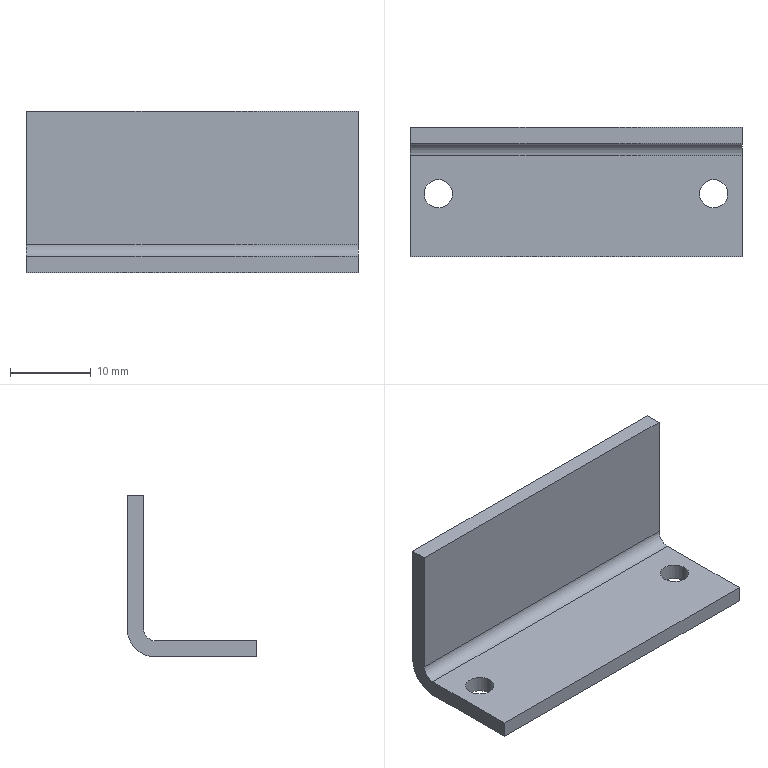Part | SolidWorks | features BaseBody 1 | 1 solid | 14 faces | box 41 x 16 x 20 mm | volume 2662 mm3 | plane 8 | cylinder 6 | commonest cylinder face diameters 3.5 x4 3 x1 7 x1
STEP:
#1=CARTESIAN_POINT('',(-15.25,-0.2,0.));
#2=VERTEX_POINT('',#1);
#3=CARTESIAN_POINT('',(-18.75,-0.2,0.));
#4=VERTEX_POINT('',#3);
#5=CARTESIAN_POINT('',(-17.,-0.2,0.));
#6=DIRECTION('',(0.,0.,-1.));
#7=DIRECTION('',(-1.,0.,0.));
#8=AXIS2_PLACEMENT_3D('',#5,#6,#7);
#9=CIRCLE('',#8,1.75);
#10=EDGE_CURVE('',#2,#4,#9,.T.);
#11=ORIENTED_EDGE('',*,*,#10,.F.);
#12=CARTESIAN_POINT('',(-15.25,-0.2,-2.));
#13=VERTEX_POINT('',#12);
#14=CARTESIAN_POINT('',(-15.25,-0.2,8.));
#15=DIRECTION('',(0.,0.,-1.));
#16=VECTOR('',#15,1000.);
#17=LINE('',#14,#16);
#18=EDGE_CURVE('',#2,#13,#17,.T.);
#19=ORIENTED_EDGE('',*,*,#18,.T.);
#20=CARTESIAN_POINT('',(-18.75,-0.2,-2.));
#21=VERTEX_POINT('',#20);
#22=CARTESIAN_POINT('',(-17.,-0.2,-2.));
#23=DIRECTION('',(0.,0.,1.));
#24=DIRECTION('',(-1.,0.,0.));
#25=AXIS2_PLACEMENT_3D('',#22,#23,#24);
#26=CIRCLE('',#25,1.75);
#27=EDGE_CURVE('',#21,#13,#26,.T.);
#28=ORIENTED_EDGE('',*,*,#27,.F.);
#29=CARTESIAN_POINT('',(-18.75,-0.2,8.));
#30=DIRECTION('',(0.,0.,-1.));
#31=VECTOR('',#30,1000.);
#32=LINE('',#29,#31);
#33=EDGE_CURVE('',#4,#21,#32,.T.);
#34=ORIENTED_EDGE('',*,*,#33,.F.);
#35=EDGE_LOOP('',(#11,#19,#28,#34));
#36=FACE_OUTER_BOUND('',#35,.T.);
#37=CARTESIAN_POINT('',(-17.,-0.2,8.));
#38=DIRECTION('',(0.,0.,-1.));
#39=DIRECTION('',(-1.,0.,0.));
#40=AXIS2_PLACEMENT_3D('',#37,#38,#39);
#41=CYLINDRICAL_SURFACE('',#40,1.75);
#42=ADVANCED_FACE('',(#36),#41,.F.);
#43=CARTESIAN_POINT('',(18.75,-0.2,0.));
#44=VERTEX_POINT('',#43);
#45=CARTESIAN_POINT('',(15.25,-0.2,0.));
#46=VERTEX_POINT('',#45);
#47=CARTESIAN_POINT('',(17.,-0.2,0.));
#48=DIRECTION('',(0.,0.,-1.));
#49=DIRECTION('',(-1.,0.,0.));
#50=AXIS2_PLACEMENT_3D('',#47,#48,#49);
#51=CIRCLE('',#50,1.75);
#52=EDGE_CURVE('',#44,#46,#51,.T.);
#53=ORIENTED_EDGE('',*,*,#52,.F.);
#54=CARTESIAN_POINT('',(18.75,-0.2,-2.));
#55=VERTEX_POINT('',#54);
#56=CARTESIAN_POINT('',(18.75,-0.2,8.));
#57=DIRECTION('',(0.,0.,-1.));
#58=VECTOR('',#57,1000.);
#59=LINE('',#56,#58);
#60=EDGE_CURVE('',#44,#55,#59,.T.);
#61=ORIENTED_EDGE('',*,*,#60,.T.);
#62=CARTESIAN_POINT('',(15.25,-0.2,-2.));
#63=VERTEX_POINT('',#62);
#64=CARTESIAN_POINT('',(17.,-0.2,-2.));
#65=DIRECTION('',(0.,0.,1.));
#66=DIRECTION('',(-1.,0.,0.));
#67=AXIS2_PLACEMENT_3D('',#64,#65,#66);
#68=CIRCLE('',#67,1.75);
#69=EDGE_CURVE('',#63,#55,#68,.T.);
#70=ORIENTED_EDGE('',*,*,#69,.F.);
#71=CARTESIAN_POINT('',(15.25,-0.2,8.));
#72=DIRECTION('',(0.,0.,-1.));
#73=VECTOR('',#72,1000.);
#74=LINE('',#71,#73);
#75=EDGE_CURVE('',#46,#63,#74,.T.);
#76=ORIENTED_EDGE('',*,*,#75,.F.);
#77=EDGE_LOOP('',(#53,#61,#70,#76));
#78=FACE_OUTER_BOUND('',#77,.T.);
#79=CARTESIAN_POINT('',(17.,-0.2,8.));
#80=DIRECTION('',(0.,0.,-1.));
#81=DIRECTION('',(-1.,0.,0.));
#82=AXIS2_PLACEMENT_3D('',#79,#80,#81);
#83=CYLINDRICAL_SURFACE('',#82,1.75);
#84=ADVANCED_FACE('',(#78),#83,.F.);
#85=CARTESIAN_POINT('',(-20.5,8.,1.5));
#86=VERTEX_POINT('',#85);
#87=CARTESIAN_POINT('',(-20.5,8.,18.));
#88=VERTEX_POINT('',#87);
#89=CARTESIAN_POINT('',(-20.5,8.,0.));
#90=DIRECTION('',(0.,0.,1.));
#91=VECTOR('',#90,1000.);
#92=LINE('',#89,#91);
#93=EDGE_CURVE('',#86,#88,#92,.T.);
#94=ORIENTED_EDGE('',*,*,#93,.T.);
#95=CARTESIAN_POINT('',(20.5,8.,18.));
#96=VERTEX_POINT('',#95);
#97=CARTESIAN_POINT('',(0.,8.,18.));
#98=DIRECTION('',(1.,0.,0.));
#99=VECTOR('',#98,1000.);
#100=LINE('',#97,#99);
#101=EDGE_CURVE('',#88,#96,#100,.T.);
#102=ORIENTED_EDGE('',*,*,#101,.T.);
#103=CARTESIAN_POINT('',(20.5,8.,1.5));
#104=VERTEX_POINT('',#103);
#105=CARTESIAN_POINT('',(20.5,8.,0.));
#106=DIRECTION('',(0.,0.,-1.));
#107=VECTOR('',#106,1000.);
#108=LINE('',#105,#107);
#109=EDGE_CURVE('',#96,#104,#108,.T.);
#110=ORIENTED_EDGE('',*,*,#109,.T.);
#111=CARTESIAN_POINT('',(0.,8.,1.5));
#112=DIRECTION('',(-1.,0.,0.));
#113=VECTOR('',#112,1000.);
#114=LINE('',#111,#113);
#115=EDGE_CURVE('',#104,#86,#114,.T.);
#116=ORIENTED_EDGE('',*,*,#115,.T.);
#117=EDGE_LOOP('',(#94,#102,#110,#116));
#118=FACE_OUTER_BOUND('',#117,.T.);
#119=CARTESIAN_POINT('',(0.,8.,0.));
#120=DIRECTION('',(0.,1.,0.));
#121=DIRECTION('',(0.,0.,1.));
#122=AXIS2_PLACEMENT_3D('',#119,#120,#121);
#123=PLANE('',#122);
#124=ADVANCED_FACE('',(#118),#123,.T.);
#125=ORIENTED_EDGE('',*,*,#101,.F.);
#126=CARTESIAN_POINT('',(-20.5,6.,18.));
#127=VERTEX_POINT('',#126);
#128=CARTESIAN_POINT('',(-20.5,8.,18.));
#129=DIRECTION('',(0.,-1.,0.));
#130=VECTOR('',#129,1000.);
#131=LINE('',#128,#130);
#132=EDGE_CURVE('',#88,#127,#131,.T.);
#133=ORIENTED_EDGE('',*,*,#132,.T.);
#134=CARTESIAN_POINT('',(20.5,6.,18.));
#135=VERTEX_POINT('',#134);
#136=CARTESIAN_POINT('',(-20.5,6.,18.));
#137=DIRECTION('',(1.,0.,0.));
#138=VECTOR('',#137,1000.);
#139=LINE('',#136,#138);
#140=EDGE_CURVE('',#127,#135,#139,.T.);
#141=ORIENTED_EDGE('',*,*,#140,.T.);
#142=CARTESIAN_POINT('',(20.5,8.,18.));
#143=DIRECTION('',(0.,1.,0.));
#144=VECTOR('',#143,1000.);
#145=LINE('',#142,#144);
#146=EDGE_CURVE('',#135,#96,#145,.T.);
#147=ORIENTED_EDGE('',*,*,#146,.T.);
#148=EDGE_LOOP('',(#125,#133,#141,#147));
#149=FACE_OUTER_BOUND('',#148,.T.);
#150=CARTESIAN_POINT('',(-20.5,8.,18.));
#151=DIRECTION('',(0.,0.,1.));
#152=DIRECTION('',(0.,-1.,0.));
#153=AXIS2_PLACEMENT_3D('',#150,#151,#152);
#154=PLANE('',#153);
#155=ADVANCED_FACE('',(#149),#154,.T.);
#156=CARTESIAN_POINT('',(-20.5,6.,1.5));
#157=VERTEX_POINT('',#156);
#158=CARTESIAN_POINT('',(-20.5,6.,0.));
#159=DIRECTION('',(0.,0.,1.));
#160=VECTOR('',#159,1000.);
#161=LINE('',#158,#160);
#162=EDGE_CURVE('',#157,#127,#161,.T.);
#163=ORIENTED_EDGE('',*,*,#162,.T.);
#164=ORIENTED_EDGE('',*,*,#132,.F.);
#165=ORIENTED_EDGE('',*,*,#93,.F.);
#166=CARTESIAN_POINT('',(-20.5,4.5,-2.));
#167=VERTEX_POINT('',#166);
#168=CARTESIAN_POINT('',(-20.5,4.5,1.5));
#169=DIRECTION('',(1.,0.,0.));
#170=DIRECTION('',(0.,0.,1.));
#171=AXIS2_PLACEMENT_3D('',#168,#169,#170);
#172=CIRCLE('',#171,3.5);
#173=EDGE_CURVE('',#167,#86,#172,.T.);
#174=ORIENTED_EDGE('',*,*,#173,.F.);
#175=CARTESIAN_POINT('',(-20.5,-8.,-2.));
#176=VERTEX_POINT('',#175);
#177=CARTESIAN_POINT('',(-20.5,0.,-2.));
#178=DIRECTION('',(0.,1.,0.));
#179=VECTOR('',#178,1000.);
#180=LINE('',#177,#179);
#181=EDGE_CURVE('',#176,#167,#180,.T.);
#182=ORIENTED_EDGE('',*,*,#181,.F.);
#183=CARTESIAN_POINT('',(-20.5,-8.,0.));
#184=VERTEX_POINT('',#183);
#185=CARTESIAN_POINT('',(-20.5,-8.,-2.));
#186=DIRECTION('',(0.,0.,1.));
#187=VECTOR('',#186,1000.);
#188=LINE('',#185,#187);
#189=EDGE_CURVE('',#176,#184,#188,.T.);
#190=ORIENTED_EDGE('',*,*,#189,.T.);
#191=CARTESIAN_POINT('',(-20.5,4.5,0.));
#192=VERTEX_POINT('',#191);
#193=CARTESIAN_POINT('',(-20.5,-8.,0.));
#194=DIRECTION('',(0.,1.,0.));
#195=VECTOR('',#194,1000.);
#196=LINE('',#193,#195);
#197=EDGE_CURVE('',#184,#192,#196,.T.);
#198=ORIENTED_EDGE('',*,*,#197,.T.);
#199=CARTESIAN_POINT('',(-20.5,4.5,1.5));
#200=DIRECTION('',(-1.,0.,0.));
#201=DIRECTION('',(0.,0.,1.));
#202=AXIS2_PLACEMENT_3D('',#199,#200,#201);
#203=CIRCLE('',#202,1.5);
#204=EDGE_CURVE('',#157,#192,#203,.T.);
#205=ORIENTED_EDGE('',*,*,#204,.F.);
#206=EDGE_LOOP('',(#163,#164,#165,#174,#182,#190,#198,#205));
#207=FACE_OUTER_BOUND('',#206,.T.);
#208=CARTESIAN_POINT('',(-20.5,8.,0.));
#209=DIRECTION('',(-1.,0.,0.));
#210=DIRECTION('',(0.,0.,1.));
#211=AXIS2_PLACEMENT_3D('',#208,#209,#210);
#212=PLANE('',#211);
#213=ADVANCED_FACE('',(#207),#212,.T.);
#214=ORIENTED_EDGE('',*,*,#115,.F.);
#215=CARTESIAN_POINT('',(20.5,4.5,-2.));
#216=VERTEX_POINT('',#215);
#217=CARTESIAN_POINT('',(20.5,4.5,1.5));
#218=DIRECTION('',(-1.,0.,0.));
#219=DIRECTION('',(0.,0.,1.));
#220=AXIS2_PLACEMENT_3D('',#217,#218,#219);
#221=CIRCLE('',#220,3.5);
#222=EDGE_CURVE('',#104,#216,#221,.T.);
#223=ORIENTED_EDGE('',*,*,#222,.T.);
#224=CARTESIAN_POINT('',(-20.5,4.5,-2.));
#225=DIRECTION('',(-1.,0.,0.));
#226=VECTOR('',#225,1000.);
#227=LINE('',#224,#226);
#228=EDGE_CURVE('',#216,#167,#227,.T.);
#229=ORIENTED_EDGE('',*,*,#228,.T.);
#230=ORIENTED_EDGE('',*,*,#173,.T.);
#231=EDGE_LOOP('',(#214,#223,#229,#230));
#232=FACE_OUTER_BOUND('',#231,.T.);
#233=CARTESIAN_POINT('',(-20.5,4.5,1.5));
#234=DIRECTION('',(-1.,0.,0.));
#235=DIRECTION('',(0.,0.,1.));
#236=AXIS2_PLACEMENT_3D('',#233,#234,#235);
#237=CYLINDRICAL_SURFACE('',#236,3.5);
#238=ADVANCED_FACE('',(#232),#237,.T.);
#239=ORIENTED_EDGE('',*,*,#109,.F.);
#240=ORIENTED_EDGE('',*,*,#146,.F.);
#241=CARTESIAN_POINT('',(20.5,6.,1.5));
#242=VERTEX_POINT('',#241);
#243=CARTESIAN_POINT('',(20.5,6.,18.));
#244=DIRECTION('',(0.,0.,-1.));
#245=VECTOR('',#244,1000.);
#246=LINE('',#243,#245);
#247=EDGE_CURVE('',#135,#242,#246,.T.);
#248=ORIENTED_EDGE('',*,*,#247,.T.);
#249=CARTESIAN_POINT('',(20.5,4.5,0.));
#250=VERTEX_POINT('',#249);
#251=CARTESIAN_POINT('',(20.5,4.5,1.5));
#252=DIRECTION('',(-1.,0.,0.));
#253=DIRECTION('',(0.,0.,1.));
#254=AXIS2_PLACEMENT_3D('',#251,#252,#253);
#255=CIRCLE('',#254,1.5);
#256=EDGE_CURVE('',#242,#250,#255,.T.);
#257=ORIENTED_EDGE('',*,*,#256,.T.);
#258=CARTESIAN_POINT('',(20.5,-8.,0.));
#259=VERTEX_POINT('',#258);
#260=CARTESIAN_POINT('',(20.5,-8.,0.));
#261=DIRECTION('',(0.,-1.,0.));
#262=VECTOR('',#261,1000.);
#263=LINE('',#260,#262);
#264=EDGE_CURVE('',#250,#259,#263,.T.);
#265=ORIENTED_EDGE('',*,*,#264,.T.);
#266=CARTESIAN_POINT('',(20.5,-8.,-2.));
#267=VERTEX_POINT('',#266);
#268=CARTESIAN_POINT('',(20.5,-8.,-2.));
#269=DIRECTION('',(0.,0.,-1.));
#270=VECTOR('',#269,1000.);
#271=LINE('',#268,#270);
#272=EDGE_CURVE('',#259,#267,#271,.T.);
#273=ORIENTED_EDGE('',*,*,#272,.T.);
#274=CARTESIAN_POINT('',(20.5,0.,-2.));
#275=DIRECTION('',(0.,-1.,0.));
#276=VECTOR('',#275,1000.);
#277=LINE('',#274,#276);
#278=EDGE_CURVE('',#216,#267,#277,.T.);
#279=ORIENTED_EDGE('',*,*,#278,.F.);
#280=ORIENTED_EDGE('',*,*,#222,.F.);
#281=EDGE_LOOP('',(#239,#240,#248,#257,#265,#273,#279,#280));
#282=FACE_OUTER_BOUND('',#281,.T.);
#283=CARTESIAN_POINT('',(20.5,8.,18.));
#284=DIRECTION('',(1.,0.,0.));
#285=DIRECTION('',(0.,0.,-1.));
#286=AXIS2_PLACEMENT_3D('',#283,#284,#285);
#287=PLANE('',#286);
#288=ADVANCED_FACE('',(#282),#287,.T.);
#289=ORIENTED_EDGE('',*,*,#247,.F.);
#290=ORIENTED_EDGE('',*,*,#140,.F.);
#291=ORIENTED_EDGE('',*,*,#162,.F.);
#292=CARTESIAN_POINT('',(0.,6.,1.5));
#293=DIRECTION('',(-1.,0.,0.));
#294=VECTOR('',#293,1000.);
#295=LINE('',#292,#294);
#296=EDGE_CURVE('',#242,#157,#295,.T.);
#297=ORIENTED_EDGE('',*,*,#296,.F.);
#298=EDGE_LOOP('',(#289,#290,#291,#297));
#299=FACE_OUTER_BOUND('',#298,.T.);
#300=CARTESIAN_POINT('',(0.,6.,0.));
#301=DIRECTION('',(0.,1.,0.));
#302=DIRECTION('',(0.,0.,1.));
#303=AXIS2_PLACEMENT_3D('',#300,#301,#302);
#304=PLANE('',#303);
#305=ADVANCED_FACE('',(#299),#304,.F.);
#306=ORIENTED_EDGE('',*,*,#278,.T.);
#307=CARTESIAN_POINT('',(0.,-8.,-2.));
#308=DIRECTION('',(-1.,0.,0.));
#309=VECTOR('',#308,1000.);
#310=LINE('',#307,#309);
#311=EDGE_CURVE('',#267,#176,#310,.T.);
#312=ORIENTED_EDGE('',*,*,#311,.T.);
#313=ORIENTED_EDGE('',*,*,#181,.T.);
#314=ORIENTED_EDGE('',*,*,#228,.F.);
#315=EDGE_LOOP('',(#306,#312,#313,#314));
#316=FACE_OUTER_BOUND('',#315,.T.);
#317=ORIENTED_EDGE('',*,*,#27,.T.);
#318=CARTESIAN_POINT('',(-17.,-0.2,-2.));
#319=DIRECTION('',(0.,0.,1.));
#320=DIRECTION('',(-1.,0.,0.));
#321=AXIS2_PLACEMENT_3D('',#318,#319,#320);
#322=CIRCLE('',#321,1.75);
#323=EDGE_CURVE('',#13,#21,#322,.T.);
#324=ORIENTED_EDGE('',*,*,#323,.T.);
#325=EDGE_LOOP('',(#317,#324));
#326=FACE_BOUND('',#325,.T.);
#327=ORIENTED_EDGE('',*,*,#69,.T.);
#328=CARTESIAN_POINT('',(17.,-0.2,-2.));
#329=DIRECTION('',(0.,0.,1.));
#330=DIRECTION('',(-1.,0.,0.));
#331=AXIS2_PLACEMENT_3D('',#328,#329,#330);
#332=CIRCLE('',#331,1.75);
#333=EDGE_CURVE('',#55,#63,#332,.T.);
#334=ORIENTED_EDGE('',*,*,#333,.T.);
#335=EDGE_LOOP('',(#327,#334));
#336=FACE_BOUND('',#335,.T.);
#337=CARTESIAN_POINT('',(0.,0.,-2.));
#338=DIRECTION('',(0.,0.,-1.));
#339=DIRECTION('',(-1.,0.,0.));
#340=AXIS2_PLACEMENT_3D('',#337,#338,#339);
#341=PLANE('',#340);
#342=ADVANCED_FACE('',(#316,#326,#336),#341,.T.);
#343=ORIENTED_EDGE('',*,*,#256,.F.);
#344=ORIENTED_EDGE('',*,*,#296,.T.);
#345=ORIENTED_EDGE('',*,*,#204,.T.);
#346=CARTESIAN_POINT('',(-20.5,4.5,0.));
#347=DIRECTION('',(-1.,0.,0.));
#348=VECTOR('',#347,1000.);
#349=LINE('',#346,#348);
#350=EDGE_CURVE('',#250,#192,#349,.T.);
#351=ORIENTED_EDGE('',*,*,#350,.F.);
#352=EDGE_LOOP('',(#343,#344,#345,#351));
#353=FACE_OUTER_BOUND('',#352,.T.);
#354=CARTESIAN_POINT('',(-20.5,4.5,1.5));
#355=DIRECTION('',(-1.,0.,0.));
#356=DIRECTION('',(0.,0.,1.));
#357=AXIS2_PLACEMENT_3D('',#354,#355,#356);
#358=CYLINDRICAL_SURFACE('',#357,1.5);
#359=ADVANCED_FACE('',(#353),#358,.F.);
#360=ORIENTED_EDGE('',*,*,#311,.F.);
#361=ORIENTED_EDGE('',*,*,#272,.F.);
#362=CARTESIAN_POINT('',(-20.5,-8.,0.));
#363=DIRECTION('',(-1.,0.,0.));
#364=VECTOR('',#363,1000.);
#365=LINE('',#362,#364);
#366=EDGE_CURVE('',#259,#184,#365,.T.);
#367=ORIENTED_EDGE('',*,*,#366,.T.);
#368=ORIENTED_EDGE('',*,*,#189,.F.);
#369=EDGE_LOOP('',(#360,#361,#367,#368));
#370=FACE_OUTER_BOUND('',#369,.T.);
#371=CARTESIAN_POINT('',(-20.5,-8.,-2.));
#372=DIRECTION('',(0.,-1.,0.));
#373=DIRECTION('',(0.,0.,-1.));
#374=AXIS2_PLACEMENT_3D('',#371,#372,#373);
#375=PLANE('',#374);
#376=ADVANCED_FACE('',(#370),#375,.T.);
#377=ORIENTED_EDGE('',*,*,#18,.F.);
#378=CARTESIAN_POINT('',(-17.,-0.2,0.));
#379=DIRECTION('',(0.,0.,-1.));
#380=DIRECTION('',(-1.,0.,0.));
#381=AXIS2_PLACEMENT_3D('',#378,#379,#380);
#382=CIRCLE('',#381,1.75);
#383=EDGE_CURVE('',#4,#2,#382,.T.);
#384=ORIENTED_EDGE('',*,*,#383,.F.);
#385=ORIENTED_EDGE('',*,*,#33,.T.);
#386=ORIENTED_EDGE('',*,*,#323,.F.);
#387=EDGE_LOOP('',(#377,#384,#385,#386));
#388=FACE_OUTER_BOUND('',#387,.T.);
#389=CARTESIAN_POINT('',(-17.,-0.2,8.));
#390=DIRECTION('',(0.,0.,-1.));
#391=DIRECTION('',(-1.,0.,0.));
#392=AXIS2_PLACEMENT_3D('',#389,#390,#391);
#393=CYLINDRICAL_SURFACE('',#392,1.75);
#394=ADVANCED_FACE('',(#388),#393,.F.);
#395=ORIENTED_EDGE('',*,*,#60,.F.);
#396=CARTESIAN_POINT('',(17.,-0.2,0.));
#397=DIRECTION('',(0.,0.,-1.));
#398=DIRECTION('',(-1.,0.,0.));
#399=AXIS2_PLACEMENT_3D('',#396,#397,#398);
#400=CIRCLE('',#399,1.75);
#401=EDGE_CURVE('',#46,#44,#400,.T.);
#402=ORIENTED_EDGE('',*,*,#401,.F.);
#403=ORIENTED_EDGE('',*,*,#75,.T.);
#404=ORIENTED_EDGE('',*,*,#333,.F.);
#405=EDGE_LOOP('',(#395,#402,#403,#404));
#406=FACE_OUTER_BOUND('',#405,.T.);
#407=CARTESIAN_POINT('',(17.,-0.2,8.));
#408=DIRECTION('',(0.,0.,-1.));
#409=DIRECTION('',(-1.,0.,0.));
#410=AXIS2_PLACEMENT_3D('',#407,#408,#409);
#411=CYLINDRICAL_SURFACE('',#410,1.75);
#412=ADVANCED_FACE('',(#406),#411,.F.);
#413=ORIENTED_EDGE('',*,*,#197,.F.);
#414=ORIENTED_EDGE('',*,*,#366,.F.);
#415=ORIENTED_EDGE('',*,*,#264,.F.);
#416=ORIENTED_EDGE('',*,*,#350,.T.);
#417=EDGE_LOOP('',(#413,#414,#415,#416));
#418=FACE_OUTER_BOUND('',#417,.T.);
#419=ORIENTED_EDGE('',*,*,#383,.T.);
#420=ORIENTED_EDGE('',*,*,#10,.T.);
#421=EDGE_LOOP('',(#419,#420));
#422=FACE_BOUND('',#421,.T.);
#423=ORIENTED_EDGE('',*,*,#401,.T.);
#424=ORIENTED_EDGE('',*,*,#52,.T.);
#425=EDGE_LOOP('',(#423,#424));
#426=FACE_BOUND('',#425,.T.);
#427=CARTESIAN_POINT('',(0.,0.,0.));
#428=DIRECTION('',(0.,0.,-1.));
#429=DIRECTION('',(-1.,0.,0.));
#430=AXIS2_PLACEMENT_3D('',#427,#428,#429);
#431=PLANE('',#430);
#432=ADVANCED_FACE('',(#418,#422,#426),#431,.F.);
#433=CLOSED_SHELL('',(#42,#84,#124,#155,#213,#238,#288,#305,#342,#359,#376,#394,#412,#432));
#434=MANIFOLD_SOLID_BREP('',#433);
#435=CARTESIAN_POINT('',(0.,0.,0.));
#436=DIRECTION('',(0.,0.,1.));
#437=DIRECTION('',(1.,0.,0.));
#438=AXIS2_PLACEMENT_3D('',#435,#436,#437);
#439=(LENGTH_UNIT()NAMED_UNIT(*)SI_UNIT(.MILLI.,.METRE.));
#440=UNCERTAINTY_MEASURE_WITH_UNIT(LENGTH_MEASURE(0.00001),#439,'','');
#441=(NAMED_UNIT(*)PLANE_ANGLE_UNIT()SI_UNIT($,.RADIAN.));
#442=(NAMED_UNIT(*)SI_UNIT($,.STERADIAN.)SOLID_ANGLE_UNIT());
#443=(GEOMETRIC_REPRESENTATION_CONTEXT(3)GLOBAL_UNCERTAINTY_ASSIGNED_CONTEXT((#440))GLOBAL_UNIT_ASSIGNED_CONTEXT((#439,#441,#442))REPRESENTATION_CONTEXT('',''));
#444=ADVANCED_BREP_SHAPE_REPRESENTATION('',(#434,#438),#443);